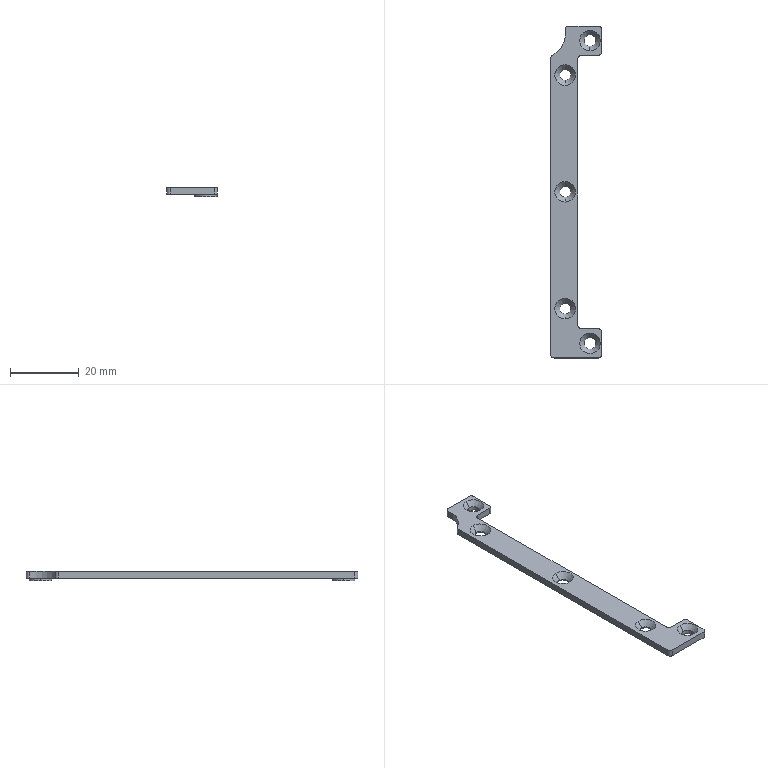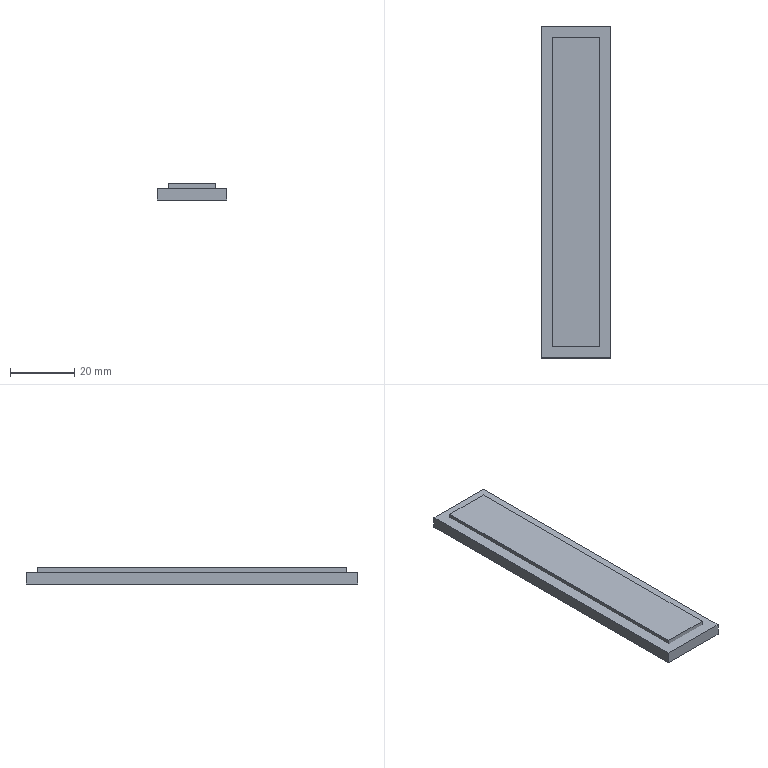CAM job | NX | 3-axis milling, drilling | part box 14.723 x 96.5 x 2.7 mm | stock box 21.723 x 103.5 x 5 mm
Tools:
number,name,description,diameter,corner_radius,flute_length,length,flutes
6,D6,Milling Tool-5 Parameters,6.0,0.0,50.0,75.0,2
4,D4,Milling Tool-5 Parameters,4.0,0.0,50.0,75.0,2
2,D2,Milling Tool-5 Parameters,2.0,0.0,50.0,75.0,2
7,D6A45,Milling Tool-5 Parameters,6.0,0.0,50.0,75.0,2
Operations:
program,operation,operation_type,tool,method,geometry_group,spindle_rpm,surface_speed,feed_per_tooth,feed_cut,feed_plunge,cut_length_mm,path_length_mm,cut_time_min,machine_time_min
1,FLOOR_WALL,VolumeBased25DMillingOperation,D6,METHOD,A,9500.0,179.0,0.0789,1500.0,100.0,907.319,961.319,0.6049,0.6103
1,DRILLING,Operation,D6A45,METHOD,A,5000.0,94.0,0.025,250.0,0.0,30.0,225.621,0.12,0.1396
1,CAVITY_MILL,CavityMilling,D4,METHOD,A,9500.0,119.0,0.1316,2500.0,1000.0,5838.735,6002.941,2.323,2.339
1,CAVITY_MILL_COPY,CavityMilling,D4,METHOD,A,9500.0,119.0,0.0632,1200.0,1000.0,246.652,310.052,0.2037,0.21
1,CAVITY_MILL_COPY_1,CavityMilling,D2,METHOD,A,9500.0,59.0,0.0632,1200.0,1000.0,180.668,911.605,0.1056,0.1787
1,HOLE_MILLING,CylinderMilling,D2,METHOD,A,9500.0,59.0,0.0658,1250.0,100.0,312.619,714.158,0.2501,0.2902
1,PLANAR_MILL,PlanarMilling,D6A45,METHOD,A,9500.0,179.0,0.0658,1250.0,100.0,242.624,301.624,0.1941,0.2
2,FLOOR_WALL_COPY,VolumeBased25DMillingOperation,D6,METHOD,B,9500.0,179.0,0.0789,1500.0,100.0,3246.597,3556.677,2.164,2.195
2,FLOOR_WALL_1,VolumeBased25DMillingOperation,D4,METHOD,B,9500.0,119.0,0.1316,2500.0,1000.0,1312.98,1435.829,0.5293,0.5416
2,FLOOR_WALL_1_COPY,VolumeBased25DMillingOperation,D4,METHOD,B,9500.0,119.0,0.0632,1200.0,1000.0,584.178,1250.658,0.4911,0.5577
2,PLANAR_MILL_COPY,PlanarMilling,D6A45,METHOD,B,9500.0,179.0,0.0658,1250.0,100.0,83.209,410.075,0.0666,0.0993
2,PLANAR_MILL_COPY_COPY,PlanarMilling,D6A45,METHOD,B,9500.0,179.0,0.0658,1250.0,100.0,276.371,732.833,0.2211,0.2667